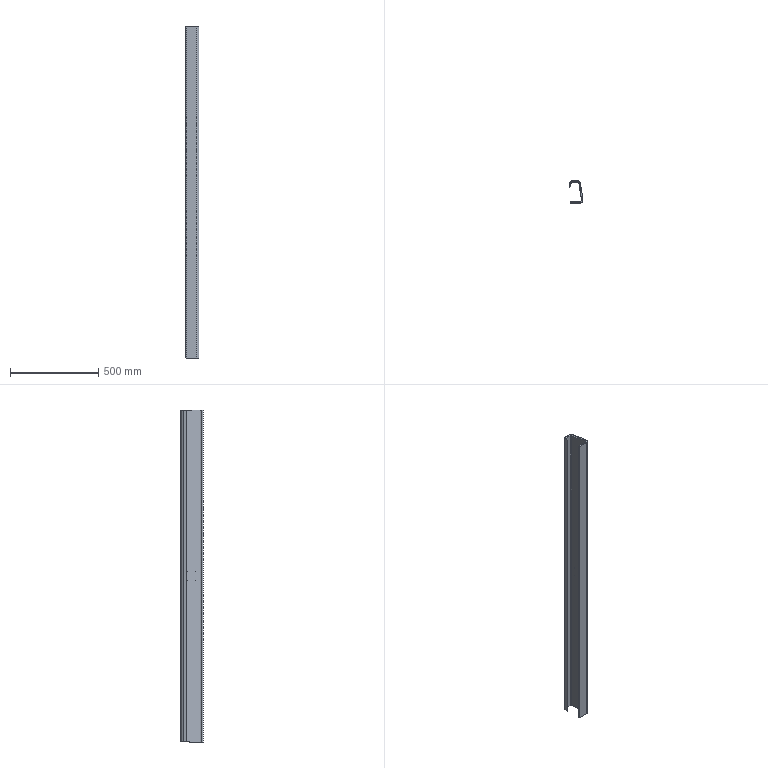Part | STEP file | 1 solid | 45 faces | box 78.969 x 125 x 1880 mm | volume 3813981 mm3 | plane 27 | cylinder 14 | cone 4 | commonest cylinder face diameters 4.2 x8 16 x3 32 x3